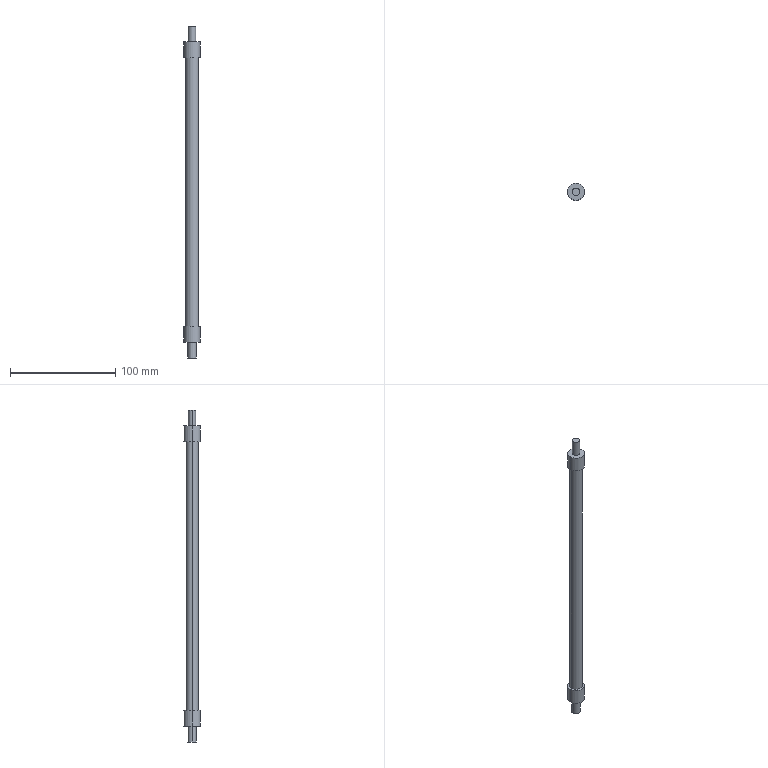Part | SolidWorks | features ICE 4, Extrusion 1 | 1 solid | 16 faces | box 16 x 16 x 315 mm | volume 36203 mm3 | cylinder 10 | plane 6 | commonest cylinder face diameters 16 x4 7 x2 8 x2 12 x2
STEP:
#1=CARTESIAN_POINT('',(3.5,0.,315.));
#2=VERTEX_POINT('',#1);
#3=CARTESIAN_POINT('',(-3.5,0.,315.));
#4=VERTEX_POINT('',#3);
#5=CARTESIAN_POINT('',(0.,0.,315.));
#6=DIRECTION('',(0.,0.,1.));
#7=DIRECTION('',(1.,0.,0.));
#8=AXIS2_PLACEMENT_3D('',#5,#6,#7);
#9=CIRCLE('',#8,3.5);
#10=EDGE_CURVE('',#2,#4,#9,.T.);
#11=ORIENTED_EDGE('',*,*,#10,.F.);
#12=CARTESIAN_POINT('',(3.5,0.,300.));
#13=VERTEX_POINT('',#12);
#14=CARTESIAN_POINT('',(3.5,0.,315.));
#15=DIRECTION('',(0.,0.,-1.));
#16=VECTOR('',#15,1000.);
#17=LINE('',#14,#16);
#18=EDGE_CURVE('',#2,#13,#17,.T.);
#19=ORIENTED_EDGE('',*,*,#18,.T.);
#20=CARTESIAN_POINT('',(-3.5,0.,300.));
#21=VERTEX_POINT('',#20);
#22=CARTESIAN_POINT('',(0.,0.,300.));
#23=DIRECTION('',(0.,0.,1.));
#24=DIRECTION('',(1.,0.,0.));
#25=AXIS2_PLACEMENT_3D('',#22,#23,#24);
#26=CIRCLE('',#25,3.5);
#27=EDGE_CURVE('',#13,#21,#26,.T.);
#28=ORIENTED_EDGE('',*,*,#27,.T.);
#29=CARTESIAN_POINT('',(-3.5,0.,315.));
#30=DIRECTION('',(0.,0.,-1.));
#31=VECTOR('',#30,1000.);
#32=LINE('',#29,#31);
#33=EDGE_CURVE('',#4,#21,#32,.T.);
#34=ORIENTED_EDGE('',*,*,#33,.F.);
#35=EDGE_LOOP('',(#11,#19,#28,#34));
#36=FACE_OUTER_BOUND('',#35,.T.);
#37=CARTESIAN_POINT('',(0.,0.,315.));
#38=DIRECTION('',(0.,0.,-1.));
#39=DIRECTION('',(-1.,0.,0.));
#40=AXIS2_PLACEMENT_3D('',#37,#38,#39);
#41=CYLINDRICAL_SURFACE('',#40,3.5);
#42=ADVANCED_FACE('',(#36),#41,.T.);
#43=CARTESIAN_POINT('',(8.,0.,300.));
#44=VERTEX_POINT('',#43);
#45=CARTESIAN_POINT('',(-8.,0.,300.));
#46=VERTEX_POINT('',#45);
#47=CARTESIAN_POINT('',(0.,0.,300.));
#48=DIRECTION('',(0.,0.,1.));
#49=DIRECTION('',(1.,0.,0.));
#50=AXIS2_PLACEMENT_3D('',#47,#48,#49);
#51=CIRCLE('',#50,8.);
#52=EDGE_CURVE('',#44,#46,#51,.T.);
#53=ORIENTED_EDGE('',*,*,#52,.F.);
#54=CARTESIAN_POINT('',(8.,0.,285.));
#55=VERTEX_POINT('',#54);
#56=CARTESIAN_POINT('',(8.,0.,300.));
#57=DIRECTION('',(0.,0.,-1.));
#58=VECTOR('',#57,1000.);
#59=LINE('',#56,#58);
#60=EDGE_CURVE('',#44,#55,#59,.T.);
#61=ORIENTED_EDGE('',*,*,#60,.T.);
#62=CARTESIAN_POINT('',(-8.,0.,285.));
#63=VERTEX_POINT('',#62);
#64=CARTESIAN_POINT('',(0.,0.,285.));
#65=DIRECTION('',(0.,0.,1.));
#66=DIRECTION('',(1.,0.,0.));
#67=AXIS2_PLACEMENT_3D('',#64,#65,#66);
#68=CIRCLE('',#67,8.);
#69=EDGE_CURVE('',#55,#63,#68,.T.);
#70=ORIENTED_EDGE('',*,*,#69,.T.);
#71=CARTESIAN_POINT('',(-8.,0.,300.));
#72=DIRECTION('',(0.,0.,-1.));
#73=VECTOR('',#72,1000.);
#74=LINE('',#71,#73);
#75=EDGE_CURVE('',#46,#63,#74,.T.);
#76=ORIENTED_EDGE('',*,*,#75,.F.);
#77=EDGE_LOOP('',(#53,#61,#70,#76));
#78=FACE_OUTER_BOUND('',#77,.T.);
#79=CARTESIAN_POINT('',(0.,0.,300.));
#80=DIRECTION('',(0.,0.,-1.));
#81=DIRECTION('',(-1.,0.,0.));
#82=AXIS2_PLACEMENT_3D('',#79,#80,#81);
#83=CYLINDRICAL_SURFACE('',#82,8.);
#84=ADVANCED_FACE('',(#78),#83,.T.);
#85=CARTESIAN_POINT('',(6.,0.,285.));
#86=VERTEX_POINT('',#85);
#87=CARTESIAN_POINT('',(-6.,0.,285.));
#88=VERTEX_POINT('',#87);
#89=CARTESIAN_POINT('',(0.,0.,285.));
#90=DIRECTION('',(0.,0.,1.));
#91=DIRECTION('',(1.,0.,0.));
#92=AXIS2_PLACEMENT_3D('',#89,#90,#91);
#93=CIRCLE('',#92,6.);
#94=EDGE_CURVE('',#86,#88,#93,.T.);
#95=ORIENTED_EDGE('',*,*,#94,.F.);
#96=CARTESIAN_POINT('',(6.,0.,30.));
#97=VERTEX_POINT('',#96);
#98=CARTESIAN_POINT('',(6.,0.,285.));
#99=DIRECTION('',(0.,0.,-1.));
#100=VECTOR('',#99,1000.);
#101=LINE('',#98,#100);
#102=EDGE_CURVE('',#86,#97,#101,.T.);
#103=ORIENTED_EDGE('',*,*,#102,.T.);
#104=CARTESIAN_POINT('',(-6.,0.,30.));
#105=VERTEX_POINT('',#104);
#106=CARTESIAN_POINT('',(0.,0.,30.));
#107=DIRECTION('',(0.,0.,-1.));
#108=DIRECTION('',(-1.,0.,0.));
#109=AXIS2_PLACEMENT_3D('',#106,#107,#108);
#110=CIRCLE('',#109,6.);
#111=EDGE_CURVE('',#105,#97,#110,.T.);
#112=ORIENTED_EDGE('',*,*,#111,.F.);
#113=CARTESIAN_POINT('',(-6.,0.,285.));
#114=DIRECTION('',(0.,0.,-1.));
#115=VECTOR('',#114,1000.);
#116=LINE('',#113,#115);
#117=EDGE_CURVE('',#88,#105,#116,.T.);
#118=ORIENTED_EDGE('',*,*,#117,.F.);
#119=EDGE_LOOP('',(#95,#103,#112,#118));
#120=FACE_OUTER_BOUND('',#119,.T.);
#121=CARTESIAN_POINT('',(0.,0.,285.));
#122=DIRECTION('',(0.,0.,-1.));
#123=DIRECTION('',(-1.,0.,0.));
#124=AXIS2_PLACEMENT_3D('',#121,#122,#123);
#125=CYLINDRICAL_SURFACE('',#124,6.);
#126=ADVANCED_FACE('',(#120),#125,.T.);
#127=CARTESIAN_POINT('',(-8.,0.,30.));
#128=VERTEX_POINT('',#127);
#129=CARTESIAN_POINT('',(8.,0.,30.));
#130=VERTEX_POINT('',#129);
#131=CARTESIAN_POINT('',(0.,0.,30.));
#132=DIRECTION('',(0.,0.,-1.));
#133=DIRECTION('',(-1.,0.,0.));
#134=AXIS2_PLACEMENT_3D('',#131,#132,#133);
#135=CIRCLE('',#134,8.);
#136=EDGE_CURVE('',#128,#130,#135,.T.);
#137=ORIENTED_EDGE('',*,*,#136,.T.);
#138=CARTESIAN_POINT('',(8.,0.,15.));
#139=VERTEX_POINT('',#138);
#140=CARTESIAN_POINT('',(8.,0.,30.));
#141=DIRECTION('',(0.,0.,-1.));
#142=VECTOR('',#141,1000.);
#143=LINE('',#140,#142);
#144=EDGE_CURVE('',#130,#139,#143,.T.);
#145=ORIENTED_EDGE('',*,*,#144,.T.);
#146=CARTESIAN_POINT('',(-8.,0.,15.));
#147=VERTEX_POINT('',#146);
#148=CARTESIAN_POINT('',(0.,0.,15.));
#149=DIRECTION('',(0.,0.,-1.));
#150=DIRECTION('',(-1.,0.,0.));
#151=AXIS2_PLACEMENT_3D('',#148,#149,#150);
#152=CIRCLE('',#151,8.);
#153=EDGE_CURVE('',#147,#139,#152,.T.);
#154=ORIENTED_EDGE('',*,*,#153,.F.);
#155=CARTESIAN_POINT('',(-8.,0.,30.));
#156=DIRECTION('',(0.,0.,-1.));
#157=VECTOR('',#156,1000.);
#158=LINE('',#155,#157);
#159=EDGE_CURVE('',#128,#147,#158,.T.);
#160=ORIENTED_EDGE('',*,*,#159,.F.);
#161=EDGE_LOOP('',(#137,#145,#154,#160));
#162=FACE_OUTER_BOUND('',#161,.T.);
#163=CARTESIAN_POINT('',(0.,0.,30.));
#164=DIRECTION('',(0.,0.,-1.));
#165=DIRECTION('',(-1.,0.,0.));
#166=AXIS2_PLACEMENT_3D('',#163,#164,#165);
#167=CYLINDRICAL_SURFACE('',#166,8.);
#168=ADVANCED_FACE('',(#162),#167,.T.);
#169=CARTESIAN_POINT('',(4.,0.,15.));
#170=VERTEX_POINT('',#169);
#171=CARTESIAN_POINT('',(-4.,0.,15.));
#172=VERTEX_POINT('',#171);
#173=CARTESIAN_POINT('',(0.,0.,15.));
#174=DIRECTION('',(0.,0.,1.));
#175=DIRECTION('',(1.,0.,0.));
#176=AXIS2_PLACEMENT_3D('',#173,#174,#175);
#177=CIRCLE('',#176,4.);
#178=EDGE_CURVE('',#170,#172,#177,.T.);
#179=ORIENTED_EDGE('',*,*,#178,.F.);
#180=CARTESIAN_POINT('',(4.,0.,0.));
#181=VERTEX_POINT('',#180);
#182=CARTESIAN_POINT('',(4.,0.,15.));
#183=DIRECTION('',(0.,0.,-1.));
#184=VECTOR('',#183,1000.);
#185=LINE('',#182,#184);
#186=EDGE_CURVE('',#170,#181,#185,.T.);
#187=ORIENTED_EDGE('',*,*,#186,.T.);
#188=CARTESIAN_POINT('',(-4.,0.,0.));
#189=VERTEX_POINT('',#188);
#190=CARTESIAN_POINT('',(0.,0.,0.));
#191=DIRECTION('',(0.,0.,1.));
#192=DIRECTION('',(1.,0.,0.));
#193=AXIS2_PLACEMENT_3D('',#190,#191,#192);
#194=CIRCLE('',#193,4.);
#195=EDGE_CURVE('',#181,#189,#194,.T.);
#196=ORIENTED_EDGE('',*,*,#195,.T.);
#197=CARTESIAN_POINT('',(-4.,0.,15.));
#198=DIRECTION('',(0.,0.,-1.));
#199=VECTOR('',#198,1000.);
#200=LINE('',#197,#199);
#201=EDGE_CURVE('',#172,#189,#200,.T.);
#202=ORIENTED_EDGE('',*,*,#201,.F.);
#203=EDGE_LOOP('',(#179,#187,#196,#202));
#204=FACE_OUTER_BOUND('',#203,.T.);
#205=CARTESIAN_POINT('',(0.,0.,15.));
#206=DIRECTION('',(0.,0.,-1.));
#207=DIRECTION('',(-1.,0.,0.));
#208=AXIS2_PLACEMENT_3D('',#205,#206,#207);
#209=CYLINDRICAL_SURFACE('',#208,4.);
#210=ADVANCED_FACE('',(#204),#209,.T.);
#211=ORIENTED_EDGE('',*,*,#186,.F.);
#212=CARTESIAN_POINT('',(0.,0.,15.));
#213=DIRECTION('',(0.,0.,1.));
#214=DIRECTION('',(1.,0.,0.));
#215=AXIS2_PLACEMENT_3D('',#212,#213,#214);
#216=CIRCLE('',#215,4.);
#217=EDGE_CURVE('',#172,#170,#216,.T.);
#218=ORIENTED_EDGE('',*,*,#217,.F.);
#219=ORIENTED_EDGE('',*,*,#201,.T.);
#220=CARTESIAN_POINT('',(0.,0.,0.));
#221=DIRECTION('',(0.,0.,1.));
#222=DIRECTION('',(1.,0.,0.));
#223=AXIS2_PLACEMENT_3D('',#220,#221,#222);
#224=CIRCLE('',#223,4.);
#225=EDGE_CURVE('',#189,#181,#224,.T.);
#226=ORIENTED_EDGE('',*,*,#225,.T.);
#227=EDGE_LOOP('',(#211,#218,#219,#226));
#228=FACE_OUTER_BOUND('',#227,.T.);
#229=CARTESIAN_POINT('',(0.,0.,15.));
#230=DIRECTION('',(0.,0.,-1.));
#231=DIRECTION('',(-1.,0.,0.));
#232=AXIS2_PLACEMENT_3D('',#229,#230,#231);
#233=CYLINDRICAL_SURFACE('',#232,4.);
#234=ADVANCED_FACE('',(#228),#233,.T.);
#235=ORIENTED_EDGE('',*,*,#225,.F.);
#236=ORIENTED_EDGE('',*,*,#195,.F.);
#237=EDGE_LOOP('',(#235,#236));
#238=FACE_OUTER_BOUND('',#237,.T.);
#239=CARTESIAN_POINT('',(0.,0.,0.));
#240=DIRECTION('',(0.,0.,1.));
#241=DIRECTION('',(1.,0.,0.));
#242=AXIS2_PLACEMENT_3D('',#239,#240,#241);
#243=PLANE('',#242);
#244=ADVANCED_FACE('',(#238),#243,.F.);
#245=ORIENTED_EDGE('',*,*,#217,.T.);
#246=ORIENTED_EDGE('',*,*,#178,.T.);
#247=EDGE_LOOP('',(#245,#246));
#248=FACE_BOUND('',#247,.T.);
#249=ORIENTED_EDGE('',*,*,#153,.T.);
#250=CARTESIAN_POINT('',(0.,0.,15.));
#251=DIRECTION('',(0.,0.,-1.));
#252=DIRECTION('',(-1.,0.,0.));
#253=AXIS2_PLACEMENT_3D('',#250,#251,#252);
#254=CIRCLE('',#253,8.);
#255=EDGE_CURVE('',#139,#147,#254,.T.);
#256=ORIENTED_EDGE('',*,*,#255,.T.);
#257=EDGE_LOOP('',(#249,#256));
#258=FACE_OUTER_BOUND('',#257,.T.);
#259=CARTESIAN_POINT('',(0.,0.,15.));
#260=DIRECTION('',(0.,0.,1.));
#261=DIRECTION('',(1.,0.,0.));
#262=AXIS2_PLACEMENT_3D('',#259,#260,#261);
#263=PLANE('',#262);
#264=ADVANCED_FACE('',(#248,#258),#263,.F.);
#265=ORIENTED_EDGE('',*,*,#144,.F.);
#266=CARTESIAN_POINT('',(0.,0.,30.));
#267=DIRECTION('',(0.,0.,-1.));
#268=DIRECTION('',(-1.,0.,0.));
#269=AXIS2_PLACEMENT_3D('',#266,#267,#268);
#270=CIRCLE('',#269,8.);
#271=EDGE_CURVE('',#130,#128,#270,.T.);
#272=ORIENTED_EDGE('',*,*,#271,.T.);
#273=ORIENTED_EDGE('',*,*,#159,.T.);
#274=ORIENTED_EDGE('',*,*,#255,.F.);
#275=EDGE_LOOP('',(#265,#272,#273,#274));
#276=FACE_OUTER_BOUND('',#275,.T.);
#277=CARTESIAN_POINT('',(0.,0.,30.));
#278=DIRECTION('',(0.,0.,-1.));
#279=DIRECTION('',(-1.,0.,0.));
#280=AXIS2_PLACEMENT_3D('',#277,#278,#279);
#281=CYLINDRICAL_SURFACE('',#280,8.);
#282=ADVANCED_FACE('',(#276),#281,.T.);
#283=ORIENTED_EDGE('',*,*,#111,.T.);
#284=CARTESIAN_POINT('',(0.,0.,30.));
#285=DIRECTION('',(0.,0.,-1.));
#286=DIRECTION('',(-1.,0.,0.));
#287=AXIS2_PLACEMENT_3D('',#284,#285,#286);
#288=CIRCLE('',#287,6.);
#289=EDGE_CURVE('',#97,#105,#288,.T.);
#290=ORIENTED_EDGE('',*,*,#289,.T.);
#291=EDGE_LOOP('',(#283,#290));
#292=FACE_BOUND('',#291,.T.);
#293=ORIENTED_EDGE('',*,*,#136,.F.);
#294=ORIENTED_EDGE('',*,*,#271,.F.);
#295=EDGE_LOOP('',(#293,#294));
#296=FACE_OUTER_BOUND('',#295,.T.);
#297=CARTESIAN_POINT('',(0.,0.,30.));
#298=DIRECTION('',(0.,0.,-1.));
#299=DIRECTION('',(-1.,0.,0.));
#300=AXIS2_PLACEMENT_3D('',#297,#298,#299);
#301=PLANE('',#300);
#302=ADVANCED_FACE('',(#292,#296),#301,.F.);
#303=ORIENTED_EDGE('',*,*,#102,.F.);
#304=CARTESIAN_POINT('',(0.,0.,285.));
#305=DIRECTION('',(0.,0.,1.));
#306=DIRECTION('',(1.,0.,0.));
#307=AXIS2_PLACEMENT_3D('',#304,#305,#306);
#308=CIRCLE('',#307,6.);
#309=EDGE_CURVE('',#88,#86,#308,.T.);
#310=ORIENTED_EDGE('',*,*,#309,.F.);
#311=ORIENTED_EDGE('',*,*,#117,.T.);
#312=ORIENTED_EDGE('',*,*,#289,.F.);
#313=EDGE_LOOP('',(#303,#310,#311,#312));
#314=FACE_OUTER_BOUND('',#313,.T.);
#315=CARTESIAN_POINT('',(0.,0.,285.));
#316=DIRECTION('',(0.,0.,-1.));
#317=DIRECTION('',(-1.,0.,0.));
#318=AXIS2_PLACEMENT_3D('',#315,#316,#317);
#319=CYLINDRICAL_SURFACE('',#318,6.);
#320=ADVANCED_FACE('',(#314),#319,.T.);
#321=ORIENTED_EDGE('',*,*,#60,.F.);
#322=CARTESIAN_POINT('',(0.,0.,300.));
#323=DIRECTION('',(0.,0.,1.));
#324=DIRECTION('',(1.,0.,0.));
#325=AXIS2_PLACEMENT_3D('',#322,#323,#324);
#326=CIRCLE('',#325,8.);
#327=EDGE_CURVE('',#46,#44,#326,.T.);
#328=ORIENTED_EDGE('',*,*,#327,.F.);
#329=ORIENTED_EDGE('',*,*,#75,.T.);
#330=CARTESIAN_POINT('',(0.,0.,285.));
#331=DIRECTION('',(0.,0.,1.));
#332=DIRECTION('',(1.,0.,0.));
#333=AXIS2_PLACEMENT_3D('',#330,#331,#332);
#334=CIRCLE('',#333,8.);
#335=EDGE_CURVE('',#63,#55,#334,.T.);
#336=ORIENTED_EDGE('',*,*,#335,.T.);
#337=EDGE_LOOP('',(#321,#328,#329,#336));
#338=FACE_OUTER_BOUND('',#337,.T.);
#339=CARTESIAN_POINT('',(0.,0.,300.));
#340=DIRECTION('',(0.,0.,-1.));
#341=DIRECTION('',(-1.,0.,0.));
#342=AXIS2_PLACEMENT_3D('',#339,#340,#341);
#343=CYLINDRICAL_SURFACE('',#342,8.);
#344=ADVANCED_FACE('',(#338),#343,.T.);
#345=CARTESIAN_POINT('',(0.,0.,300.));
#346=DIRECTION('',(0.,0.,1.));
#347=DIRECTION('',(1.,0.,0.));
#348=AXIS2_PLACEMENT_3D('',#345,#346,#347);
#349=CIRCLE('',#348,3.5);
#350=EDGE_CURVE('',#21,#13,#349,.T.);
#351=ORIENTED_EDGE('',*,*,#350,.F.);
#352=ORIENTED_EDGE('',*,*,#27,.F.);
#353=EDGE_LOOP('',(#351,#352));
#354=FACE_BOUND('',#353,.T.);
#355=ORIENTED_EDGE('',*,*,#327,.T.);
#356=ORIENTED_EDGE('',*,*,#52,.T.);
#357=EDGE_LOOP('',(#355,#356));
#358=FACE_OUTER_BOUND('',#357,.T.);
#359=CARTESIAN_POINT('',(0.,0.,300.));
#360=DIRECTION('',(0.,0.,1.));
#361=DIRECTION('',(1.,0.,0.));
#362=AXIS2_PLACEMENT_3D('',#359,#360,#361);
#363=PLANE('',#362);
#364=ADVANCED_FACE('',(#354,#358),#363,.T.);
#365=ORIENTED_EDGE('',*,*,#309,.T.);
#366=ORIENTED_EDGE('',*,*,#94,.T.);
#367=EDGE_LOOP('',(#365,#366));
#368=FACE_BOUND('',#367,.T.);
#369=ORIENTED_EDGE('',*,*,#335,.F.);
#370=ORIENTED_EDGE('',*,*,#69,.F.);
#371=EDGE_LOOP('',(#369,#370));
#372=FACE_OUTER_BOUND('',#371,.T.);
#373=CARTESIAN_POINT('',(0.,0.,285.));
#374=DIRECTION('',(0.,0.,1.));
#375=DIRECTION('',(1.,0.,0.));
#376=AXIS2_PLACEMENT_3D('',#373,#374,#375);
#377=PLANE('',#376);
#378=ADVANCED_FACE('',(#368,#372),#377,.F.);
#379=ORIENTED_EDGE('',*,*,#18,.F.);
#380=CARTESIAN_POINT('',(0.,0.,315.));
#381=DIRECTION('',(0.,0.,1.));
#382=DIRECTION('',(1.,0.,0.));
#383=AXIS2_PLACEMENT_3D('',#380,#381,#382);
#384=CIRCLE('',#383,3.5);
#385=EDGE_CURVE('',#4,#2,#384,.T.);
#386=ORIENTED_EDGE('',*,*,#385,.F.);
#387=ORIENTED_EDGE('',*,*,#33,.T.);
#388=ORIENTED_EDGE('',*,*,#350,.T.);
#389=EDGE_LOOP('',(#379,#386,#387,#388));
#390=FACE_OUTER_BOUND('',#389,.T.);
#391=CARTESIAN_POINT('',(0.,0.,315.));
#392=DIRECTION('',(0.,0.,-1.));
#393=DIRECTION('',(-1.,0.,0.));
#394=AXIS2_PLACEMENT_3D('',#391,#392,#393);
#395=CYLINDRICAL_SURFACE('',#394,3.5);
#396=ADVANCED_FACE('',(#390),#395,.T.);
#397=ORIENTED_EDGE('',*,*,#385,.T.);
#398=ORIENTED_EDGE('',*,*,#10,.T.);
#399=EDGE_LOOP('',(#397,#398));
#400=FACE_OUTER_BOUND('',#399,.T.);
#401=CARTESIAN_POINT('',(0.,0.,315.));
#402=DIRECTION('',(0.,0.,1.));
#403=DIRECTION('',(1.,0.,0.));
#404=AXIS2_PLACEMENT_3D('',#401,#402,#403);
#405=PLANE('',#404);
#406=ADVANCED_FACE('',(#400),#405,.T.);
#407=CLOSED_SHELL('',(#42,#84,#126,#168,#210,#234,#244,#264,#282,#302,#320,#344,#364,#378,#396,#406));
#408=MANIFOLD_SOLID_BREP('',#407);
#409=CARTESIAN_POINT('',(0.,0.,0.));
#410=DIRECTION('',(0.,0.,1.));
#411=DIRECTION('',(1.,0.,0.));
#412=AXIS2_PLACEMENT_3D('',#409,#410,#411);
#413=(LENGTH_UNIT()NAMED_UNIT(*)SI_UNIT(.MILLI.,.METRE.));
#414=UNCERTAINTY_MEASURE_WITH_UNIT(LENGTH_MEASURE(0.00001),#413,'','');
#415=(NAMED_UNIT(*)PLANE_ANGLE_UNIT()SI_UNIT($,.RADIAN.));
#416=(NAMED_UNIT(*)SI_UNIT($,.STERADIAN.)SOLID_ANGLE_UNIT());
#417=(GEOMETRIC_REPRESENTATION_CONTEXT(3)GLOBAL_UNCERTAINTY_ASSIGNED_CONTEXT((#414))GLOBAL_UNIT_ASSIGNED_CONTEXT((#413,#415,#416))REPRESENTATION_CONTEXT('',''));
#418=ADVANCED_BREP_SHAPE_REPRESENTATION('',(#408,#412),#417);